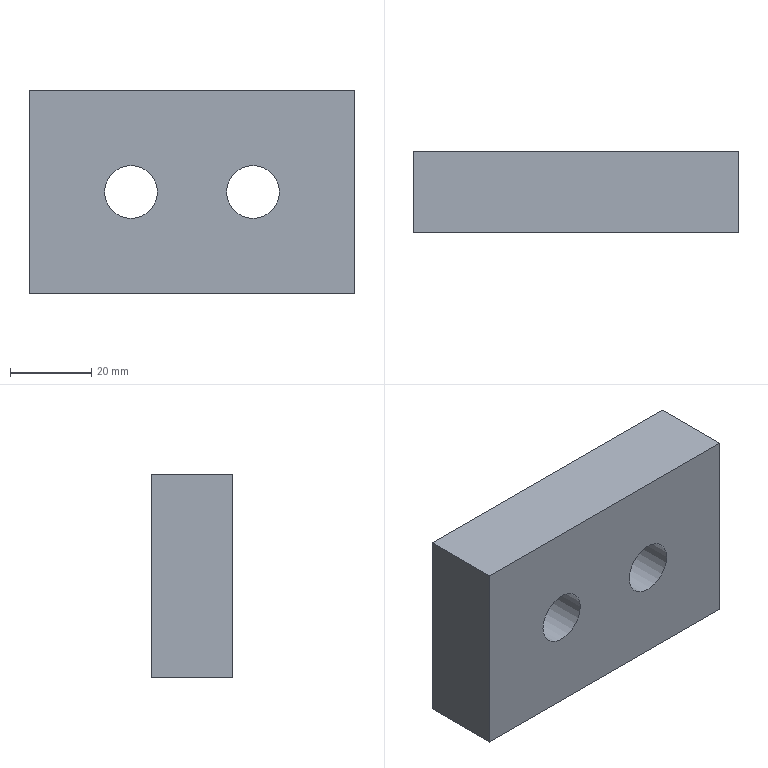Part | NX | features solid 2 | 1 solid | 12 faces | box 80 x 20 x 50 mm | volume 71062 mm3 | plane 8 | cylinder 4 | commonest cylinder face diameters 13 x2 20 x2
STEP:
#1=CARTESIAN_POINT('',(-410.,1015.,-225.));
#2=VERTEX_POINT('',#1);
#3=CARTESIAN_POINT('',(-420.,1015.,-225.));
#4=DIRECTION('',(0.,1.,0.));
#5=DIRECTION('',(1.,0.,0.));
#6=AXIS2_PLACEMENT_3D('',#3,#4,#5);
#7=CIRCLE('',#6,10.);
#8=EDGE_CURVE('',#2,#2,#7,.T.);
#9=ORIENTED_EDGE('',*,*,#8,.F.);
#10=EDGE_LOOP('',(#9));
#11=FACE_BOUND('',#10,.T.);
#12=CARTESIAN_POINT('',(-380.,1015.,-225.));
#13=VERTEX_POINT('',#12);
#14=CARTESIAN_POINT('',(-390.,1015.,-225.));
#15=DIRECTION('',(0.,1.,0.));
#16=DIRECTION('',(1.,0.,0.));
#17=AXIS2_PLACEMENT_3D('',#14,#15,#16);
#18=CIRCLE('',#17,10.);
#19=EDGE_CURVE('',#13,#13,#18,.T.);
#20=ORIENTED_EDGE('',*,*,#19,.F.);
#21=EDGE_LOOP('',(#20));
#22=FACE_BOUND('',#21,.T.);
#23=CARTESIAN_POINT('',(-365.,1015.,-250.));
#24=VERTEX_POINT('',#23);
#25=CARTESIAN_POINT('',(-365.,1015.,-200.));
#26=VERTEX_POINT('',#25);
#27=CARTESIAN_POINT('',(-365.,1015.,-225.));
#28=DIRECTION('',(0.,0.,-1.));
#29=VECTOR('',#28,1000.);
#30=LINE('',#27,#29);
#31=EDGE_CURVE('',#24,#26,#30,.F.);
#32=ORIENTED_EDGE('',*,*,#31,.F.);
#33=CARTESIAN_POINT('',(-445.,1015.,-250.));
#34=VERTEX_POINT('',#33);
#35=CARTESIAN_POINT('',(-405.,1015.,-250.));
#36=DIRECTION('',(1.,0.,0.));
#37=VECTOR('',#36,1000.);
#38=LINE('',#35,#37);
#39=EDGE_CURVE('',#24,#34,#38,.F.);
#40=ORIENTED_EDGE('',*,*,#39,.T.);
#41=CARTESIAN_POINT('',(-445.,1015.,-200.));
#42=VERTEX_POINT('',#41);
#43=CARTESIAN_POINT('',(-445.,1015.,-225.));
#44=DIRECTION('',(0.,0.,1.));
#45=VECTOR('',#44,1000.);
#46=LINE('',#43,#45);
#47=EDGE_CURVE('',#34,#42,#46,.T.);
#48=ORIENTED_EDGE('',*,*,#47,.T.);
#49=CARTESIAN_POINT('',(-405.,1015.,-200.));
#50=DIRECTION('',(1.,0.,0.));
#51=VECTOR('',#50,1000.);
#52=LINE('',#49,#51);
#53=EDGE_CURVE('',#26,#42,#52,.F.);
#54=ORIENTED_EDGE('',*,*,#53,.F.);
#55=EDGE_LOOP('',(#32,#40,#48,#54));
#56=FACE_BOUND('',#55,.T.);
#57=CARTESIAN_POINT('',(-405.,1015.,-225.));
#58=DIRECTION('',(0.,1.,0.));
#59=DIRECTION('',(-1.,0.,0.));
#60=AXIS2_PLACEMENT_3D('',#57,#58,#59);
#61=PLANE('',#60);
#62=ADVANCED_FACE('',(#11,#22,#56),#61,.T.);
#63=ORIENTED_EDGE('',*,*,#47,.F.);
#64=CARTESIAN_POINT('',(-445.,995.,-250.));
#65=VERTEX_POINT('',#64);
#66=CARTESIAN_POINT('',(-445.,1015.,-250.));
#67=DIRECTION('',(0.,1.,0.));
#68=VECTOR('',#67,1000.);
#69=LINE('',#66,#68);
#70=EDGE_CURVE('',#34,#65,#69,.F.);
#71=ORIENTED_EDGE('',*,*,#70,.T.);
#72=CARTESIAN_POINT('',(-445.,995.,-200.));
#73=VERTEX_POINT('',#72);
#74=CARTESIAN_POINT('',(-445.,995.,-225.));
#75=DIRECTION('',(0.,0.,-1.));
#76=VECTOR('',#75,1000.);
#77=LINE('',#74,#76);
#78=EDGE_CURVE('',#65,#73,#77,.F.);
#79=ORIENTED_EDGE('',*,*,#78,.T.);
#80=CARTESIAN_POINT('',(-445.,1015.,-200.));
#81=DIRECTION('',(0.,1.,0.));
#82=VECTOR('',#81,1000.);
#83=LINE('',#80,#82);
#84=EDGE_CURVE('',#42,#73,#83,.F.);
#85=ORIENTED_EDGE('',*,*,#84,.F.);
#86=EDGE_LOOP('',(#63,#71,#79,#85));
#87=FACE_BOUND('',#86,.T.);
#88=CARTESIAN_POINT('',(-445.,1015.,-225.));
#89=DIRECTION('',(-1.,0.,0.));
#90=DIRECTION('',(0.,-1.,0.));
#91=AXIS2_PLACEMENT_3D('',#88,#89,#90);
#92=PLANE('',#91);
#93=ADVANCED_FACE('',(#87),#92,.T.);
#94=CARTESIAN_POINT('',(-426.5,995.,-225.));
#95=VERTEX_POINT('',#94);
#96=CARTESIAN_POINT('',(-420.,995.,-225.));
#97=DIRECTION('',(0.,-1.,0.));
#98=DIRECTION('',(-1.,0.,0.));
#99=AXIS2_PLACEMENT_3D('',#96,#97,#98);
#100=CIRCLE('',#99,6.5);
#101=EDGE_CURVE('',#95,#95,#100,.T.);
#102=ORIENTED_EDGE('',*,*,#101,.F.);
#103=EDGE_LOOP('',(#102));
#104=FACE_BOUND('',#103,.T.);
#105=CARTESIAN_POINT('',(-396.5,995.,-225.));
#106=VERTEX_POINT('',#105);
#107=CARTESIAN_POINT('',(-390.,995.,-225.));
#108=DIRECTION('',(0.,-1.,0.));
#109=DIRECTION('',(-1.,0.,0.));
#110=AXIS2_PLACEMENT_3D('',#107,#108,#109);
#111=CIRCLE('',#110,6.5);
#112=EDGE_CURVE('',#106,#106,#111,.T.);
#113=ORIENTED_EDGE('',*,*,#112,.F.);
#114=EDGE_LOOP('',(#113));
#115=FACE_BOUND('',#114,.T.);
#116=ORIENTED_EDGE('',*,*,#78,.F.);
#117=CARTESIAN_POINT('',(-365.,995.,-250.));
#118=VERTEX_POINT('',#117);
#119=CARTESIAN_POINT('',(-405.,995.,-250.));
#120=DIRECTION('',(-1.,0.,0.));
#121=VECTOR('',#120,1000.);
#122=LINE('',#119,#121);
#123=EDGE_CURVE('',#118,#65,#122,.T.);
#124=ORIENTED_EDGE('',*,*,#123,.F.);
#125=CARTESIAN_POINT('',(-365.,995.,-200.));
#126=VERTEX_POINT('',#125);
#127=CARTESIAN_POINT('',(-365.,995.,-225.));
#128=DIRECTION('',(0.,0.,1.));
#129=VECTOR('',#128,1000.);
#130=LINE('',#127,#129);
#131=EDGE_CURVE('',#118,#126,#130,.T.);
#132=ORIENTED_EDGE('',*,*,#131,.T.);
#133=CARTESIAN_POINT('',(-405.,995.,-200.));
#134=DIRECTION('',(-1.,0.,0.));
#135=VECTOR('',#134,1000.);
#136=LINE('',#133,#135);
#137=EDGE_CURVE('',#126,#73,#136,.T.);
#138=ORIENTED_EDGE('',*,*,#137,.T.);
#139=EDGE_LOOP('',(#116,#124,#132,#138));
#140=FACE_BOUND('',#139,.T.);
#141=CARTESIAN_POINT('',(-405.,995.,-225.));
#142=DIRECTION('',(0.,1.,0.));
#143=DIRECTION('',(-1.,0.,0.));
#144=AXIS2_PLACEMENT_3D('',#141,#142,#143);
#145=PLANE('',#144);
#146=ADVANCED_FACE('',(#104,#115,#140),#145,.F.);
#147=CARTESIAN_POINT('',(-365.,1015.,-250.));
#148=DIRECTION('',(0.,-1.,0.));
#149=VECTOR('',#148,1000.);
#150=LINE('',#147,#149);
#151=EDGE_CURVE('',#24,#118,#150,.T.);
#152=ORIENTED_EDGE('',*,*,#151,.F.);
#153=ORIENTED_EDGE('',*,*,#31,.T.);
#154=CARTESIAN_POINT('',(-365.,1015.,-200.));
#155=DIRECTION('',(0.,-1.,0.));
#156=VECTOR('',#155,1000.);
#157=LINE('',#154,#156);
#158=EDGE_CURVE('',#26,#126,#157,.T.);
#159=ORIENTED_EDGE('',*,*,#158,.T.);
#160=ORIENTED_EDGE('',*,*,#131,.F.);
#161=EDGE_LOOP('',(#152,#153,#159,#160));
#162=FACE_BOUND('',#161,.T.);
#163=CARTESIAN_POINT('',(-365.,1015.,-225.));
#164=DIRECTION('',(-1.,0.,0.));
#165=DIRECTION('',(0.,-1.,0.));
#166=AXIS2_PLACEMENT_3D('',#163,#164,#165);
#167=PLANE('',#166);
#168=ADVANCED_FACE('',(#162),#167,.F.);
#169=ORIENTED_EDGE('',*,*,#137,.F.);
#170=ORIENTED_EDGE('',*,*,#158,.F.);
#171=ORIENTED_EDGE('',*,*,#53,.T.);
#172=ORIENTED_EDGE('',*,*,#84,.T.);
#173=EDGE_LOOP('',(#169,#170,#171,#172));
#174=FACE_BOUND('',#173,.T.);
#175=CARTESIAN_POINT('',(-405.,1015.,-200.));
#176=DIRECTION('',(0.,0.,-1.));
#177=DIRECTION('',(-1.,0.,0.));
#178=AXIS2_PLACEMENT_3D('',#175,#176,#177);
#179=PLANE('',#178);
#180=ADVANCED_FACE('',(#174),#179,.F.);
#181=ORIENTED_EDGE('',*,*,#123,.T.);
#182=ORIENTED_EDGE('',*,*,#70,.F.);
#183=ORIENTED_EDGE('',*,*,#39,.F.);
#184=ORIENTED_EDGE('',*,*,#151,.T.);
#185=EDGE_LOOP('',(#181,#182,#183,#184));
#186=FACE_BOUND('',#185,.T.);
#187=CARTESIAN_POINT('',(-405.,1015.,-250.));
#188=DIRECTION('',(0.,0.,-1.));
#189=DIRECTION('',(-1.,0.,0.));
#190=AXIS2_PLACEMENT_3D('',#187,#188,#189);
#191=PLANE('',#190);
#192=ADVANCED_FACE('',(#186),#191,.T.);
#193=CARTESIAN_POINT('',(-383.5,1005.,-225.));
#194=VERTEX_POINT('',#193);
#195=CARTESIAN_POINT('',(-390.,1005.,-225.));
#196=DIRECTION('',(0.,1.,0.));
#197=DIRECTION('',(1.,0.,0.));
#198=AXIS2_PLACEMENT_3D('',#195,#196,#197);
#199=CIRCLE('',#198,6.5);
#200=EDGE_CURVE('',#194,#194,#199,.T.);
#201=ORIENTED_EDGE('',*,*,#200,.F.);
#202=EDGE_LOOP('',(#201));
#203=FACE_BOUND('',#202,.T.);
#204=CARTESIAN_POINT('',(-380.,1005.,-225.));
#205=VERTEX_POINT('',#204);
#206=CARTESIAN_POINT('',(-390.,1005.,-225.));
#207=DIRECTION('',(0.,1.,0.));
#208=DIRECTION('',(1.,0.,0.));
#209=AXIS2_PLACEMENT_3D('',#206,#207,#208);
#210=CIRCLE('',#209,10.);
#211=EDGE_CURVE('',#205,#205,#210,.T.);
#212=ORIENTED_EDGE('',*,*,#211,.T.);
#213=EDGE_LOOP('',(#212));
#214=FACE_BOUND('',#213,.T.);
#215=CARTESIAN_POINT('',(-390.,1005.,-225.));
#216=DIRECTION('',(0.,-1.,0.));
#217=DIRECTION('',(1.,0.,0.));
#218=AXIS2_PLACEMENT_3D('',#215,#216,#217);
#219=PLANE('',#218);
#220=ADVANCED_FACE('',(#203,#214),#219,.F.);
#221=ORIENTED_EDGE('',*,*,#211,.F.);
#222=EDGE_LOOP('',(#221));
#223=FACE_BOUND('',#222,.T.);
#224=ORIENTED_EDGE('',*,*,#19,.T.);
#225=EDGE_LOOP('',(#224));
#226=FACE_BOUND('',#225,.T.);
#227=CARTESIAN_POINT('',(-390.,1015.,-225.));
#228=DIRECTION('',(0.,-1.,0.));
#229=DIRECTION('',(1.,0.,0.));
#230=AXIS2_PLACEMENT_3D('',#227,#228,#229);
#231=CYLINDRICAL_SURFACE('',#230,10.);
#232=ADVANCED_FACE('',(#223,#226),#231,.F.);
#233=CARTESIAN_POINT('',(-413.5,1005.,-225.));
#234=VERTEX_POINT('',#233);
#235=CARTESIAN_POINT('',(-420.,1005.,-225.));
#236=DIRECTION('',(0.,1.,0.));
#237=DIRECTION('',(1.,0.,0.));
#238=AXIS2_PLACEMENT_3D('',#235,#236,#237);
#239=CIRCLE('',#238,6.5);
#240=EDGE_CURVE('',#234,#234,#239,.T.);
#241=ORIENTED_EDGE('',*,*,#240,.F.);
#242=EDGE_LOOP('',(#241));
#243=FACE_BOUND('',#242,.T.);
#244=CARTESIAN_POINT('',(-410.,1005.,-225.));
#245=VERTEX_POINT('',#244);
#246=CARTESIAN_POINT('',(-420.,1005.,-225.));
#247=DIRECTION('',(0.,1.,0.));
#248=DIRECTION('',(1.,0.,0.));
#249=AXIS2_PLACEMENT_3D('',#246,#247,#248);
#250=CIRCLE('',#249,10.);
#251=EDGE_CURVE('',#245,#245,#250,.T.);
#252=ORIENTED_EDGE('',*,*,#251,.T.);
#253=EDGE_LOOP('',(#252));
#254=FACE_BOUND('',#253,.T.);
#255=CARTESIAN_POINT('',(-420.,1005.,-225.));
#256=DIRECTION('',(0.,-1.,0.));
#257=DIRECTION('',(1.,0.,0.));
#258=AXIS2_PLACEMENT_3D('',#255,#256,#257);
#259=PLANE('',#258);
#260=ADVANCED_FACE('',(#243,#254),#259,.F.);
#261=ORIENTED_EDGE('',*,*,#251,.F.);
#262=EDGE_LOOP('',(#261));
#263=FACE_BOUND('',#262,.T.);
#264=ORIENTED_EDGE('',*,*,#8,.T.);
#265=EDGE_LOOP('',(#264));
#266=FACE_BOUND('',#265,.T.);
#267=CARTESIAN_POINT('',(-420.,1015.,-225.));
#268=DIRECTION('',(0.,-1.,0.));
#269=DIRECTION('',(1.,0.,0.));
#270=AXIS2_PLACEMENT_3D('',#267,#268,#269);
#271=CYLINDRICAL_SURFACE('',#270,10.);
#272=ADVANCED_FACE('',(#263,#266),#271,.F.);
#273=ORIENTED_EDGE('',*,*,#200,.T.);
#274=EDGE_LOOP('',(#273));
#275=FACE_BOUND('',#274,.T.);
#276=ORIENTED_EDGE('',*,*,#112,.T.);
#277=EDGE_LOOP('',(#276));
#278=FACE_BOUND('',#277,.T.);
#279=CARTESIAN_POINT('',(-390.,1005.,-225.));
#280=DIRECTION('',(0.,-1.,0.));
#281=DIRECTION('',(1.,0.,0.));
#282=AXIS2_PLACEMENT_3D('',#279,#280,#281);
#283=CYLINDRICAL_SURFACE('',#282,6.5);
#284=ADVANCED_FACE('',(#275,#278),#283,.F.);
#285=ORIENTED_EDGE('',*,*,#240,.T.);
#286=EDGE_LOOP('',(#285));
#287=FACE_BOUND('',#286,.T.);
#288=ORIENTED_EDGE('',*,*,#101,.T.);
#289=EDGE_LOOP('',(#288));
#290=FACE_BOUND('',#289,.T.);
#291=CARTESIAN_POINT('',(-420.,1005.,-225.));
#292=DIRECTION('',(0.,-1.,0.));
#293=DIRECTION('',(1.,0.,0.));
#294=AXIS2_PLACEMENT_3D('',#291,#292,#293);
#295=CYLINDRICAL_SURFACE('',#294,6.5);
#296=ADVANCED_FACE('',(#287,#290),#295,.F.);
#297=CLOSED_SHELL('',(#62,#93,#146,#168,#180,#192,#220,#232,#260,#272,#284,#296));
#298=MANIFOLD_SOLID_BREP('',#297);
#299=(LENGTH_UNIT()NAMED_UNIT(*)SI_UNIT(.MILLI.,.METRE.));
#300=UNCERTAINTY_MEASURE_WITH_UNIT(LENGTH_MEASURE(0.00001),#299,'','');
#301=(NAMED_UNIT(*)PLANE_ANGLE_UNIT()SI_UNIT($,.RADIAN.));
#302=(NAMED_UNIT(*)SI_UNIT($,.STERADIAN.)SOLID_ANGLE_UNIT());
#303=(GEOMETRIC_REPRESENTATION_CONTEXT(3)GLOBAL_UNCERTAINTY_ASSIGNED_CONTEXT((#300))GLOBAL_UNIT_ASSIGNED_CONTEXT((#299,#301,#302))REPRESENTATION_CONTEXT('',''));
#304=ADVANCED_BREP_SHAPE_REPRESENTATION('',(#298),#303);